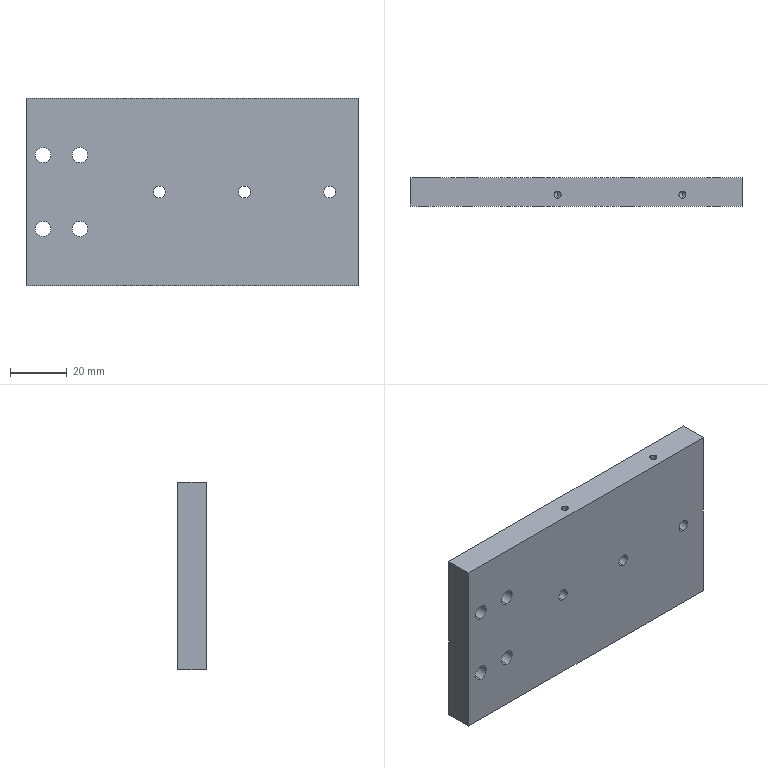Part | STEP file | 0243_220_Plate | 1 solid | 56 faces | box 117 x 10 x 66 mm | volume 74310 mm3 | cylinder 34 | cone 12 | plane 10 | commonest cylinder face diameters 4.2 x10 2.5 x8 5.5 x8 9.5 x8